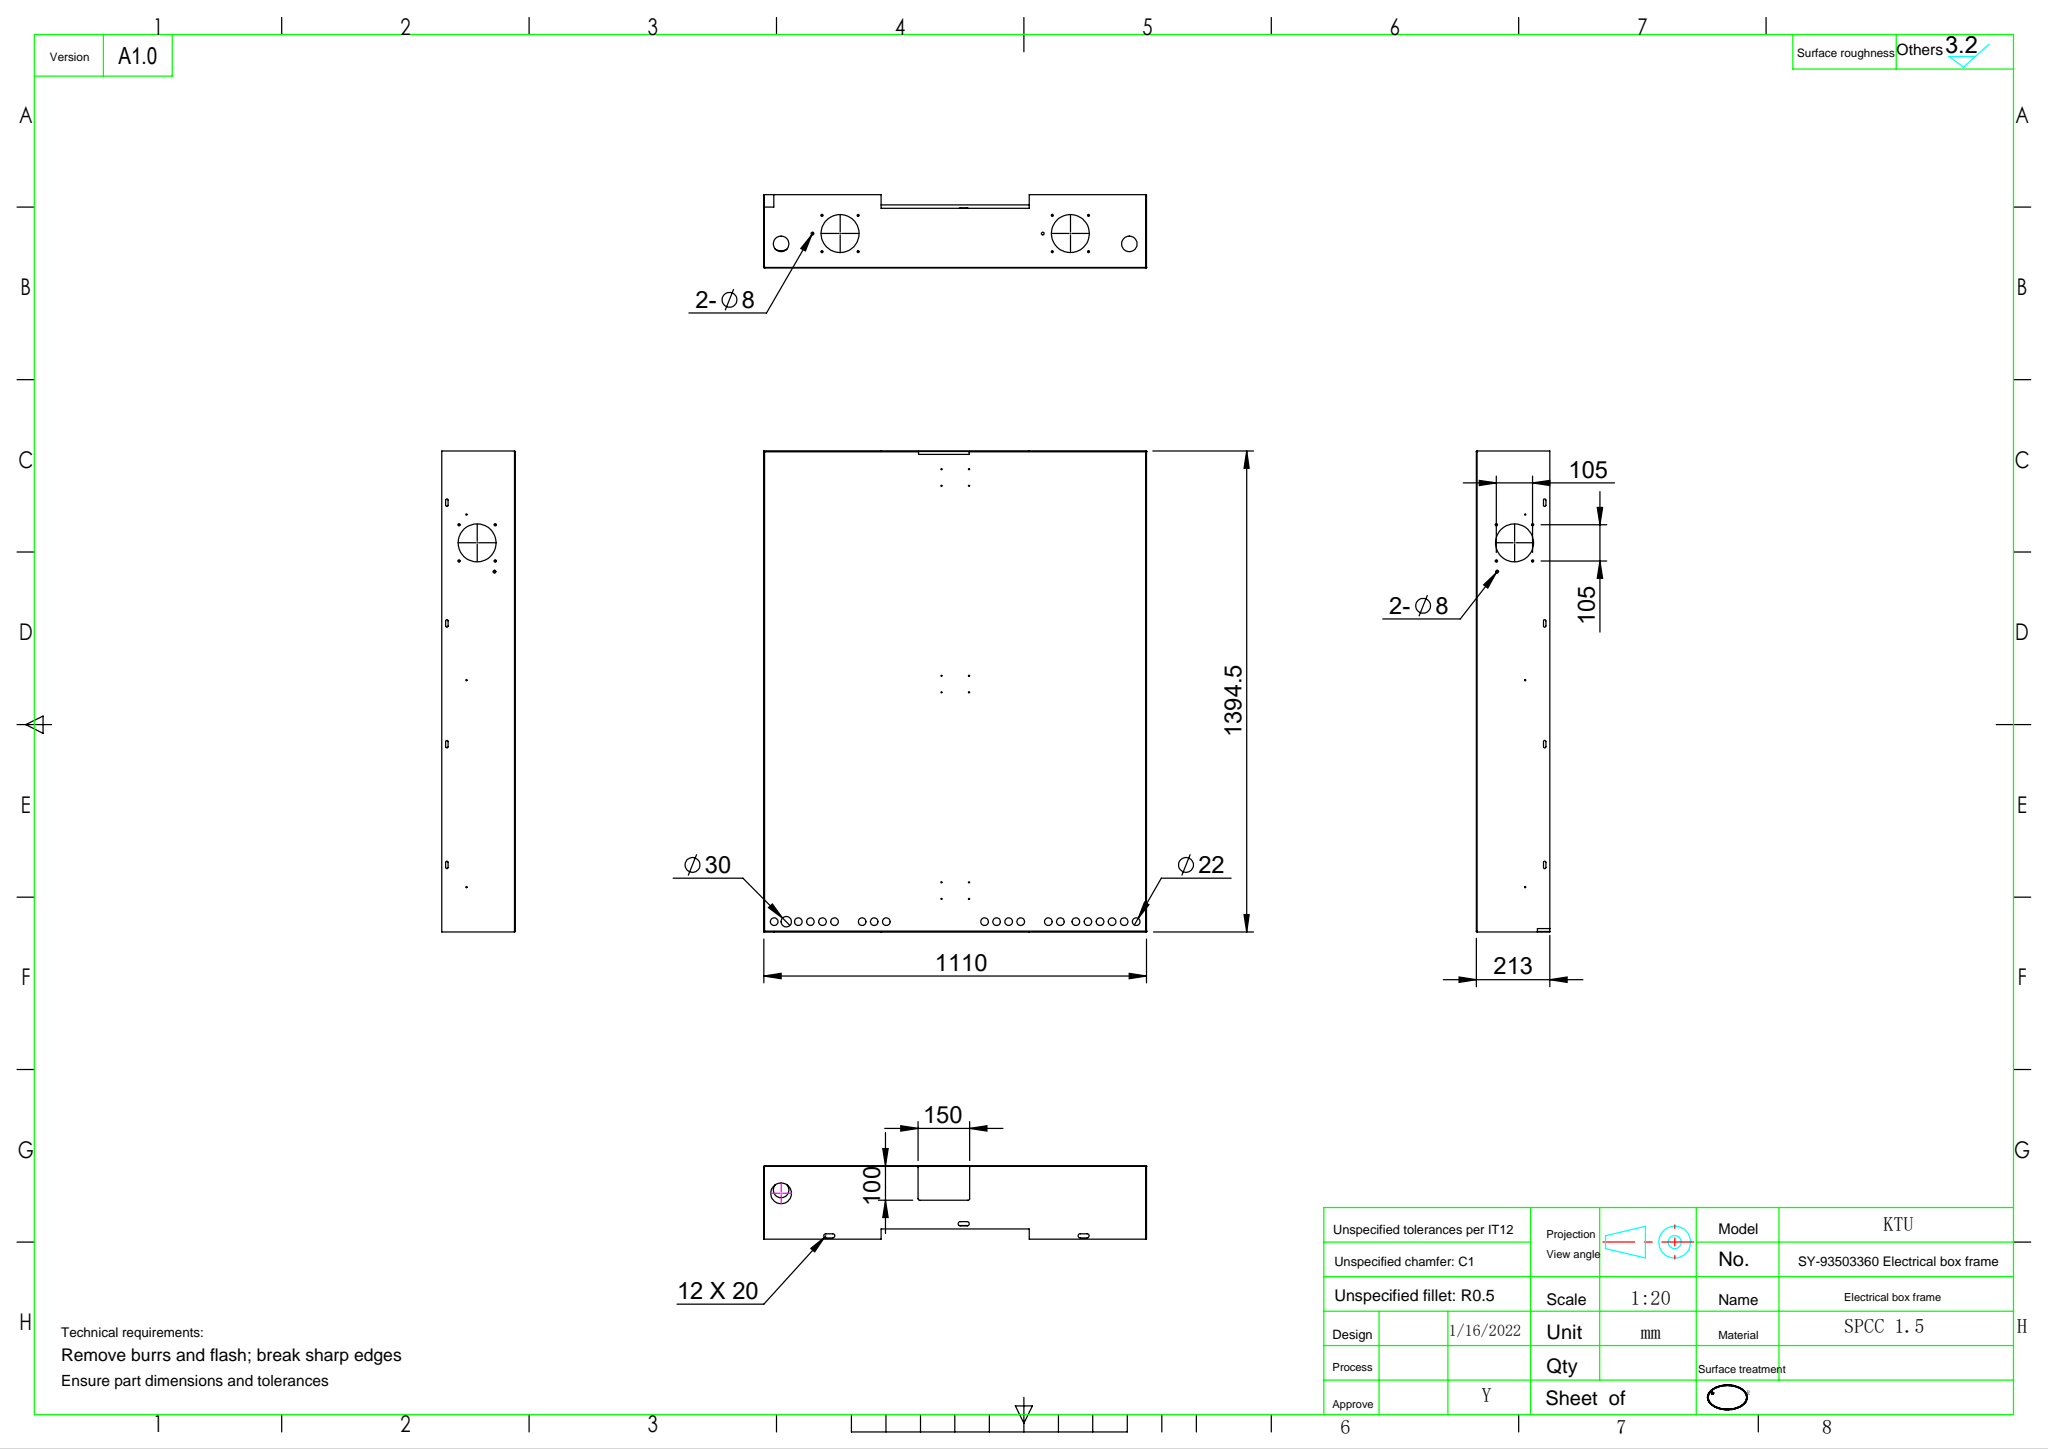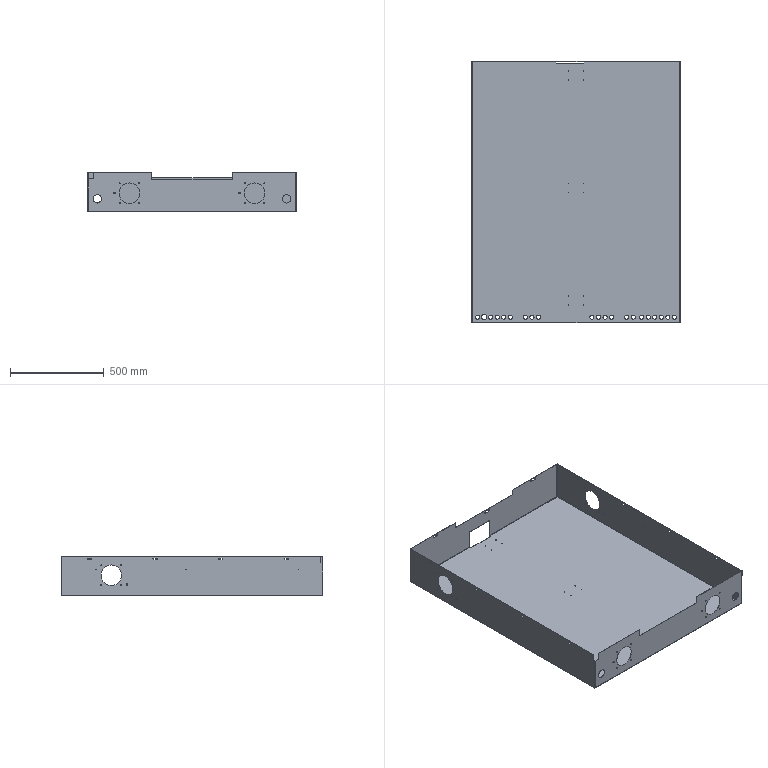Part | SolidWorks | features ICE 11, Cut 4, CornerFeat 1, EdgeFlange 1, FlatPattern 1, MirrorPattern 1, MoveFace 1, SMBaseFlange 1, SheetMetal 1 | 1 solid | 248 faces | box 1110 x 1395 x 213 mm | volume 3750548 mm3 | cylinder 168 | plane 70 | spline 10 | commonest cylinder face diameters 22 x40 3 x24 5.5 x16 6 x16 7 x16 3.42 x12